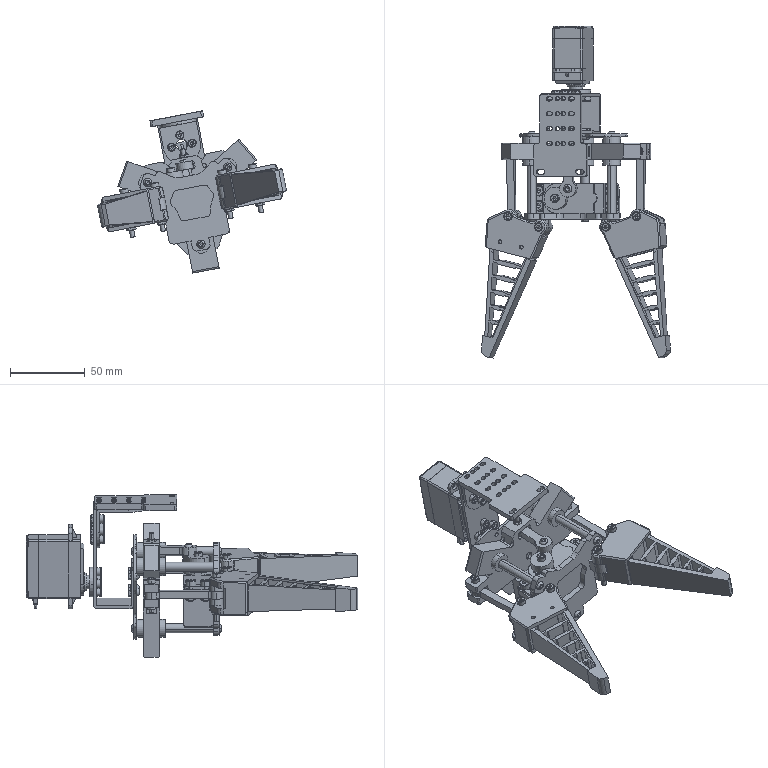Part | SolidWorks | features CompositeCurve 2 | 80 solids | 2819 faces | box 126.41 x 222.148 x 108.699 mm | volume 180398 mm3 | plane 1454 | cylinder 827 | cone 330 | torus 148 | spline 38 | sphere 22 | commonest cylinder face diameters 3 x252 6 x72 2 x54 0.4 x52 0.1 x51 4 x35